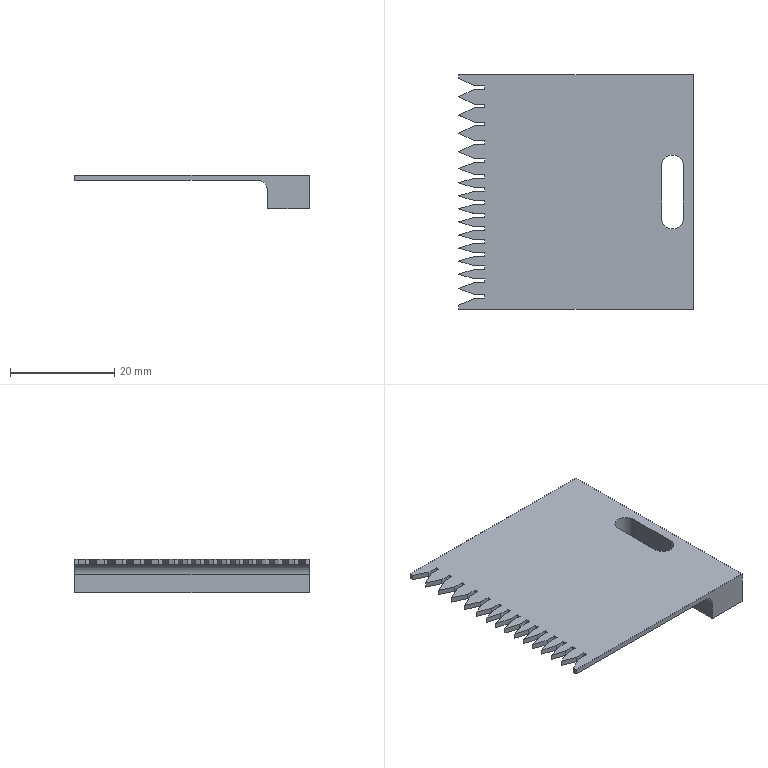Part | NX | features BREP 1 | 1 solid | 89 faces | box 45 x 45 x 6.5 mm | volume 3579 mm3 | plane 86 | cylinder 3 | commonest cylinder face diameters 4.2 x2 4 x1